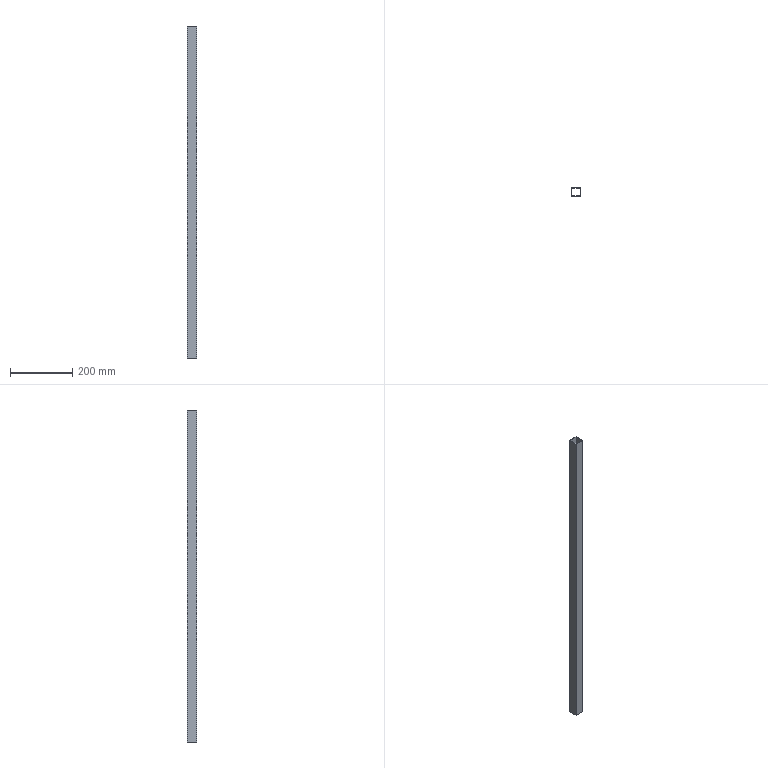Part | SolidWorks | features Extrusion 1 | 1 solid | 10 faces | box 30 x 30 x 1070 mm | volume 239680 mm3 | plane 10
STEP:
#1=CARTESIAN_POINT('',(-15.,15.,1070.));
#2=VERTEX_POINT('',#1);
#3=CARTESIAN_POINT('',(-15.,-15.,1070.));
#4=VERTEX_POINT('',#3);
#5=CARTESIAN_POINT('',(-15.,-15.,1070.));
#6=DIRECTION('',(0.,-1.,0.));
#7=VECTOR('',#6,1000.);
#8=LINE('',#5,#7);
#9=EDGE_CURVE('',#2,#4,#8,.T.);
#10=ORIENTED_EDGE('',*,*,#9,.T.);
#11=CARTESIAN_POINT('',(15.,-15.,1070.));
#12=VERTEX_POINT('',#11);
#13=CARTESIAN_POINT('',(15.,-15.,1070.));
#14=DIRECTION('',(1.,0.,0.));
#15=VECTOR('',#14,1000.);
#16=LINE('',#13,#15);
#17=EDGE_CURVE('',#4,#12,#16,.T.);
#18=ORIENTED_EDGE('',*,*,#17,.T.);
#19=CARTESIAN_POINT('',(15.,15.,1070.));
#20=VERTEX_POINT('',#19);
#21=CARTESIAN_POINT('',(15.,-15.,1070.));
#22=DIRECTION('',(0.,1.,0.));
#23=VECTOR('',#22,1000.);
#24=LINE('',#21,#23);
#25=EDGE_CURVE('',#12,#20,#24,.T.);
#26=ORIENTED_EDGE('',*,*,#25,.T.);
#27=CARTESIAN_POINT('',(15.,15.,1070.));
#28=DIRECTION('',(-1.,0.,0.));
#29=VECTOR('',#28,1000.);
#30=LINE('',#27,#29);
#31=EDGE_CURVE('',#20,#2,#30,.T.);
#32=ORIENTED_EDGE('',*,*,#31,.T.);
#33=EDGE_LOOP('',(#10,#18,#26,#32));
#34=FACE_OUTER_BOUND('',#33,.T.);
#35=CARTESIAN_POINT('',(13.,13.,1070.));
#36=VERTEX_POINT('',#35);
#37=CARTESIAN_POINT('',(-13.,13.,1070.));
#38=VERTEX_POINT('',#37);
#39=CARTESIAN_POINT('',(13.,13.,1070.));
#40=DIRECTION('',(-1.,0.,0.));
#41=VECTOR('',#40,1000.);
#42=LINE('',#39,#41);
#43=EDGE_CURVE('',#36,#38,#42,.T.);
#44=ORIENTED_EDGE('',*,*,#43,.F.);
#45=CARTESIAN_POINT('',(13.,-13.,1070.));
#46=VERTEX_POINT('',#45);
#47=CARTESIAN_POINT('',(13.,-13.,1070.));
#48=DIRECTION('',(0.,1.,0.));
#49=VECTOR('',#48,1000.);
#50=LINE('',#47,#49);
#51=EDGE_CURVE('',#46,#36,#50,.T.);
#52=ORIENTED_EDGE('',*,*,#51,.F.);
#53=CARTESIAN_POINT('',(-13.,-13.,1070.));
#54=VERTEX_POINT('',#53);
#55=CARTESIAN_POINT('',(13.,-13.,1070.));
#56=DIRECTION('',(1.,0.,0.));
#57=VECTOR('',#56,1000.);
#58=LINE('',#55,#57);
#59=EDGE_CURVE('',#54,#46,#58,.T.);
#60=ORIENTED_EDGE('',*,*,#59,.F.);
#61=CARTESIAN_POINT('',(-13.,-13.,1070.));
#62=DIRECTION('',(0.,-1.,0.));
#63=VECTOR('',#62,1000.);
#64=LINE('',#61,#63);
#65=EDGE_CURVE('',#38,#54,#64,.T.);
#66=ORIENTED_EDGE('',*,*,#65,.F.);
#67=EDGE_LOOP('',(#44,#52,#60,#66));
#68=FACE_BOUND('',#67,.T.);
#69=CARTESIAN_POINT('',(0.,0.,1070.));
#70=DIRECTION('',(0.,0.,1.));
#71=DIRECTION('',(1.,0.,0.));
#72=AXIS2_PLACEMENT_3D('',#69,#70,#71);
#73=PLANE('',#72);
#74=ADVANCED_FACE('',(#34,#68),#73,.T.);
#75=CARTESIAN_POINT('',(-15.,15.,0.));
#76=VERTEX_POINT('',#75);
#77=CARTESIAN_POINT('',(-15.,-15.,0.));
#78=VERTEX_POINT('',#77);
#79=CARTESIAN_POINT('',(-15.,-15.,0.));
#80=DIRECTION('',(0.,-1.,0.));
#81=VECTOR('',#80,1000.);
#82=LINE('',#79,#81);
#83=EDGE_CURVE('',#76,#78,#82,.T.);
#84=ORIENTED_EDGE('',*,*,#83,.F.);
#85=CARTESIAN_POINT('',(15.,15.,0.));
#86=VERTEX_POINT('',#85);
#87=CARTESIAN_POINT('',(15.,15.,0.));
#88=DIRECTION('',(-1.,0.,0.));
#89=VECTOR('',#88,1000.);
#90=LINE('',#87,#89);
#91=EDGE_CURVE('',#86,#76,#90,.T.);
#92=ORIENTED_EDGE('',*,*,#91,.F.);
#93=CARTESIAN_POINT('',(15.,-15.,0.));
#94=VERTEX_POINT('',#93);
#95=CARTESIAN_POINT('',(15.,-15.,0.));
#96=DIRECTION('',(0.,1.,0.));
#97=VECTOR('',#96,1000.);
#98=LINE('',#95,#97);
#99=EDGE_CURVE('',#94,#86,#98,.T.);
#100=ORIENTED_EDGE('',*,*,#99,.F.);
#101=CARTESIAN_POINT('',(15.,-15.,0.));
#102=DIRECTION('',(1.,0.,0.));
#103=VECTOR('',#102,1000.);
#104=LINE('',#101,#103);
#105=EDGE_CURVE('',#78,#94,#104,.T.);
#106=ORIENTED_EDGE('',*,*,#105,.F.);
#107=EDGE_LOOP('',(#84,#92,#100,#106));
#108=FACE_OUTER_BOUND('',#107,.T.);
#109=CARTESIAN_POINT('',(13.,-13.,0.));
#110=VERTEX_POINT('',#109);
#111=CARTESIAN_POINT('',(13.,13.,0.));
#112=VERTEX_POINT('',#111);
#113=CARTESIAN_POINT('',(13.,-13.,0.));
#114=DIRECTION('',(0.,1.,0.));
#115=VECTOR('',#114,1000.);
#116=LINE('',#113,#115);
#117=EDGE_CURVE('',#110,#112,#116,.T.);
#118=ORIENTED_EDGE('',*,*,#117,.T.);
#119=CARTESIAN_POINT('',(-13.,13.,0.));
#120=VERTEX_POINT('',#119);
#121=CARTESIAN_POINT('',(13.,13.,0.));
#122=DIRECTION('',(-1.,0.,0.));
#123=VECTOR('',#122,1000.);
#124=LINE('',#121,#123);
#125=EDGE_CURVE('',#112,#120,#124,.T.);
#126=ORIENTED_EDGE('',*,*,#125,.T.);
#127=CARTESIAN_POINT('',(-13.,-13.,0.));
#128=VERTEX_POINT('',#127);
#129=CARTESIAN_POINT('',(-13.,-13.,0.));
#130=DIRECTION('',(0.,-1.,0.));
#131=VECTOR('',#130,1000.);
#132=LINE('',#129,#131);
#133=EDGE_CURVE('',#120,#128,#132,.T.);
#134=ORIENTED_EDGE('',*,*,#133,.T.);
#135=CARTESIAN_POINT('',(13.,-13.,0.));
#136=DIRECTION('',(1.,0.,0.));
#137=VECTOR('',#136,1000.);
#138=LINE('',#135,#137);
#139=EDGE_CURVE('',#128,#110,#138,.T.);
#140=ORIENTED_EDGE('',*,*,#139,.T.);
#141=EDGE_LOOP('',(#118,#126,#134,#140));
#142=FACE_BOUND('',#141,.T.);
#143=CARTESIAN_POINT('',(0.,0.,0.));
#144=DIRECTION('',(0.,0.,1.));
#145=DIRECTION('',(1.,0.,0.));
#146=AXIS2_PLACEMENT_3D('',#143,#144,#145);
#147=PLANE('',#146);
#148=ADVANCED_FACE('',(#108,#142),#147,.F.);
#149=ORIENTED_EDGE('',*,*,#83,.T.);
#150=CARTESIAN_POINT('',(-15.,-15.,1070.));
#151=DIRECTION('',(0.,0.,-1.));
#152=VECTOR('',#151,1000.);
#153=LINE('',#150,#152);
#154=EDGE_CURVE('',#4,#78,#153,.T.);
#155=ORIENTED_EDGE('',*,*,#154,.F.);
#156=ORIENTED_EDGE('',*,*,#9,.F.);
#157=CARTESIAN_POINT('',(-15.,15.,1070.));
#158=DIRECTION('',(0.,0.,-1.));
#159=VECTOR('',#158,1000.);
#160=LINE('',#157,#159);
#161=EDGE_CURVE('',#2,#76,#160,.T.);
#162=ORIENTED_EDGE('',*,*,#161,.T.);
#163=EDGE_LOOP('',(#149,#155,#156,#162));
#164=FACE_OUTER_BOUND('',#163,.T.);
#165=CARTESIAN_POINT('',(-15.,-15.,1070.));
#166=DIRECTION('',(1.,0.,0.));
#167=DIRECTION('',(0.,0.,-1.));
#168=AXIS2_PLACEMENT_3D('',#165,#166,#167);
#169=PLANE('',#168);
#170=ADVANCED_FACE('',(#164),#169,.F.);
#171=ORIENTED_EDGE('',*,*,#105,.T.);
#172=CARTESIAN_POINT('',(15.,-15.,1070.));
#173=DIRECTION('',(0.,0.,-1.));
#174=VECTOR('',#173,1000.);
#175=LINE('',#172,#174);
#176=EDGE_CURVE('',#12,#94,#175,.T.);
#177=ORIENTED_EDGE('',*,*,#176,.F.);
#178=ORIENTED_EDGE('',*,*,#17,.F.);
#179=ORIENTED_EDGE('',*,*,#154,.T.);
#180=EDGE_LOOP('',(#171,#177,#178,#179));
#181=FACE_OUTER_BOUND('',#180,.T.);
#182=CARTESIAN_POINT('',(15.,-15.,1070.));
#183=DIRECTION('',(0.,1.,0.));
#184=DIRECTION('',(-1.,0.,0.));
#185=AXIS2_PLACEMENT_3D('',#182,#183,#184);
#186=PLANE('',#185);
#187=ADVANCED_FACE('',(#181),#186,.F.);
#188=ORIENTED_EDGE('',*,*,#99,.T.);
#189=CARTESIAN_POINT('',(15.,15.,1070.));
#190=DIRECTION('',(0.,0.,-1.));
#191=VECTOR('',#190,1000.);
#192=LINE('',#189,#191);
#193=EDGE_CURVE('',#20,#86,#192,.T.);
#194=ORIENTED_EDGE('',*,*,#193,.F.);
#195=ORIENTED_EDGE('',*,*,#25,.F.);
#196=ORIENTED_EDGE('',*,*,#176,.T.);
#197=EDGE_LOOP('',(#188,#194,#195,#196));
#198=FACE_OUTER_BOUND('',#197,.T.);
#199=CARTESIAN_POINT('',(15.,-15.,1070.));
#200=DIRECTION('',(-1.,0.,0.));
#201=DIRECTION('',(0.,0.,1.));
#202=AXIS2_PLACEMENT_3D('',#199,#200,#201);
#203=PLANE('',#202);
#204=ADVANCED_FACE('',(#198),#203,.F.);
#205=ORIENTED_EDGE('',*,*,#91,.T.);
#206=ORIENTED_EDGE('',*,*,#161,.F.);
#207=ORIENTED_EDGE('',*,*,#31,.F.);
#208=ORIENTED_EDGE('',*,*,#193,.T.);
#209=EDGE_LOOP('',(#205,#206,#207,#208));
#210=FACE_OUTER_BOUND('',#209,.T.);
#211=CARTESIAN_POINT('',(15.,15.,1070.));
#212=DIRECTION('',(0.,-1.,0.));
#213=DIRECTION('',(1.,0.,0.));
#214=AXIS2_PLACEMENT_3D('',#211,#212,#213);
#215=PLANE('',#214);
#216=ADVANCED_FACE('',(#210),#215,.F.);
#217=ORIENTED_EDGE('',*,*,#117,.F.);
#218=CARTESIAN_POINT('',(13.,-13.,1070.));
#219=DIRECTION('',(0.,0.,-1.));
#220=VECTOR('',#219,1000.);
#221=LINE('',#218,#220);
#222=EDGE_CURVE('',#46,#110,#221,.T.);
#223=ORIENTED_EDGE('',*,*,#222,.F.);
#224=ORIENTED_EDGE('',*,*,#51,.T.);
#225=CARTESIAN_POINT('',(13.,13.,1070.));
#226=DIRECTION('',(0.,0.,-1.));
#227=VECTOR('',#226,1000.);
#228=LINE('',#225,#227);
#229=EDGE_CURVE('',#36,#112,#228,.T.);
#230=ORIENTED_EDGE('',*,*,#229,.T.);
#231=EDGE_LOOP('',(#217,#223,#224,#230));
#232=FACE_OUTER_BOUND('',#231,.T.);
#233=CARTESIAN_POINT('',(13.,-13.,1070.));
#234=DIRECTION('',(-1.,0.,0.));
#235=DIRECTION('',(0.,0.,1.));
#236=AXIS2_PLACEMENT_3D('',#233,#234,#235);
#237=PLANE('',#236);
#238=ADVANCED_FACE('',(#232),#237,.T.);
#239=ORIENTED_EDGE('',*,*,#125,.F.);
#240=ORIENTED_EDGE('',*,*,#229,.F.);
#241=ORIENTED_EDGE('',*,*,#43,.T.);
#242=CARTESIAN_POINT('',(-13.,13.,1070.));
#243=DIRECTION('',(0.,0.,-1.));
#244=VECTOR('',#243,1000.);
#245=LINE('',#242,#244);
#246=EDGE_CURVE('',#38,#120,#245,.T.);
#247=ORIENTED_EDGE('',*,*,#246,.T.);
#248=EDGE_LOOP('',(#239,#240,#241,#247));
#249=FACE_OUTER_BOUND('',#248,.T.);
#250=CARTESIAN_POINT('',(13.,13.,1070.));
#251=DIRECTION('',(0.,-1.,0.));
#252=DIRECTION('',(1.,0.,0.));
#253=AXIS2_PLACEMENT_3D('',#250,#251,#252);
#254=PLANE('',#253);
#255=ADVANCED_FACE('',(#249),#254,.T.);
#256=ORIENTED_EDGE('',*,*,#133,.F.);
#257=ORIENTED_EDGE('',*,*,#246,.F.);
#258=ORIENTED_EDGE('',*,*,#65,.T.);
#259=CARTESIAN_POINT('',(-13.,-13.,1070.));
#260=DIRECTION('',(0.,0.,-1.));
#261=VECTOR('',#260,1000.);
#262=LINE('',#259,#261);
#263=EDGE_CURVE('',#54,#128,#262,.T.);
#264=ORIENTED_EDGE('',*,*,#263,.T.);
#265=EDGE_LOOP('',(#256,#257,#258,#264));
#266=FACE_OUTER_BOUND('',#265,.T.);
#267=CARTESIAN_POINT('',(-13.,-13.,1070.));
#268=DIRECTION('',(1.,0.,0.));
#269=DIRECTION('',(0.,0.,-1.));
#270=AXIS2_PLACEMENT_3D('',#267,#268,#269);
#271=PLANE('',#270);
#272=ADVANCED_FACE('',(#266),#271,.T.);
#273=ORIENTED_EDGE('',*,*,#139,.F.);
#274=ORIENTED_EDGE('',*,*,#263,.F.);
#275=ORIENTED_EDGE('',*,*,#59,.T.);
#276=ORIENTED_EDGE('',*,*,#222,.T.);
#277=EDGE_LOOP('',(#273,#274,#275,#276));
#278=FACE_OUTER_BOUND('',#277,.T.);
#279=CARTESIAN_POINT('',(13.,-13.,1070.));
#280=DIRECTION('',(0.,1.,0.));
#281=DIRECTION('',(0.,0.,1.));
#282=AXIS2_PLACEMENT_3D('',#279,#280,#281);
#283=PLANE('',#282);
#284=ADVANCED_FACE('',(#278),#283,.T.);
#285=CLOSED_SHELL('',(#74,#148,#170,#187,#204,#216,#238,#255,#272,#284));
#286=MANIFOLD_SOLID_BREP('',#285);
#287=CARTESIAN_POINT('',(0.,0.,0.));
#288=DIRECTION('',(0.,0.,1.));
#289=DIRECTION('',(1.,0.,0.));
#290=AXIS2_PLACEMENT_3D('',#287,#288,#289);
#291=(LENGTH_UNIT()NAMED_UNIT(*)SI_UNIT(.MILLI.,.METRE.));
#292=UNCERTAINTY_MEASURE_WITH_UNIT(LENGTH_MEASURE(0.00001),#291,'','');
#293=(NAMED_UNIT(*)PLANE_ANGLE_UNIT()SI_UNIT($,.RADIAN.));
#294=(NAMED_UNIT(*)SI_UNIT($,.STERADIAN.)SOLID_ANGLE_UNIT());
#295=(GEOMETRIC_REPRESENTATION_CONTEXT(3)GLOBAL_UNCERTAINTY_ASSIGNED_CONTEXT((#292))GLOBAL_UNIT_ASSIGNED_CONTEXT((#291,#293,#294))REPRESENTATION_CONTEXT('',''));
#296=ADVANCED_BREP_SHAPE_REPRESENTATION('',(#286,#290),#295);